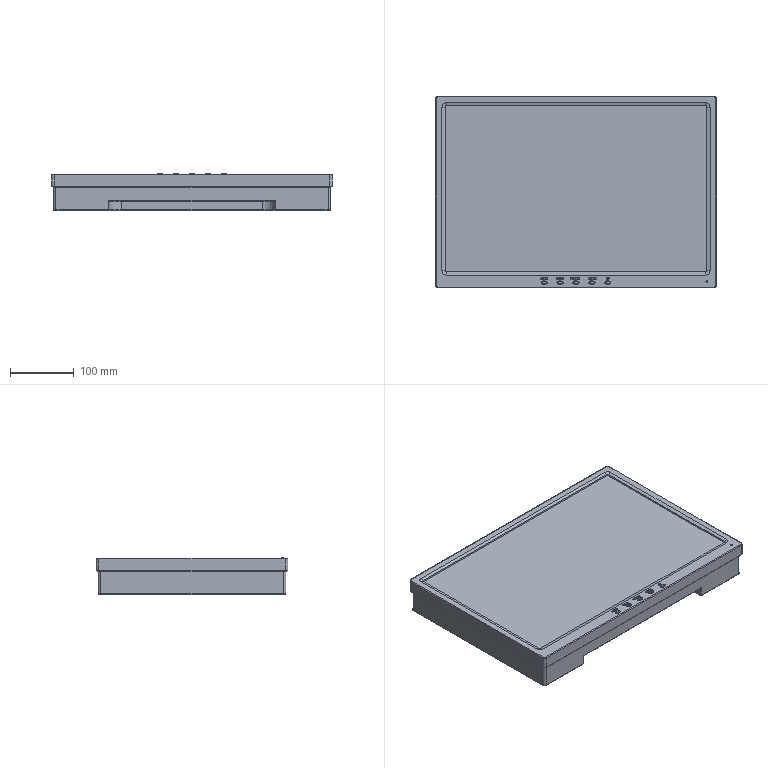Part | SolidWorks | features ICE 7, Fillet 2, Chamfer 1, Extrusion 1, HoleWzd 1, LPattern 1 | 1 solid | 442 faces | box 440 x 300 x 58 mm | volume 6630448 mm3 | plane 226 | spline 122 | cylinder 50 | torus 22 | cone 20 | sphere 2 | commonest cylinder face diameters 2 x26 3.3 x8 8 x8 4 x4 3 x2 40 x2